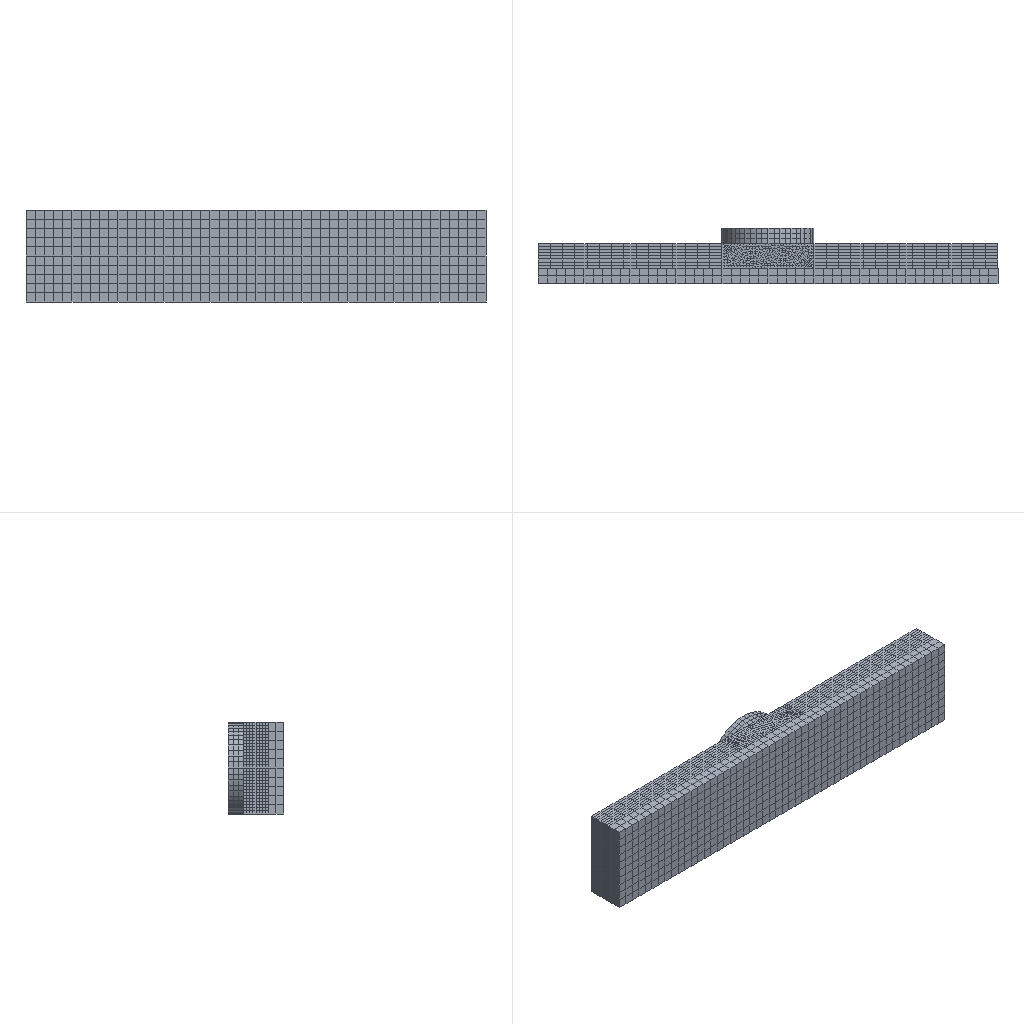Simulation study | abaqus
Set-up summary:
category,name,step,type,value,unit,region
solver,abaqus
solver,version,,,Abaqus/Explicit 2020
units,not stated in the deck,,not stated
analysis,deck,,dynamic temperature-displacement,dynamic temperature-displacement
load_step,Step-1,Step-1,dynamic temperature-displacement
load_step,requested,,,1
mesh,nodes,,,23411
mesh,elements,,,18583
element_type,C3D8RT,,solid,18583
load,load commands in deck,,count,3
bc,support commands in deck,,count,7
material,MATERIAL-1,,in results
material,STEEL,,in results
material,TOOL,,in results
check,setup vs results,,match,"per instance, exact: element labels, types and connectivity; labels of the nodes the elements use; coordinates not compared"
Abaqus input file, long lists of numbers shortened:
*Heading
** Job name: Job-1 Model name: Model-1
** Generated by: Abaqus/CAE 2020
*Preprint, echo=NO, model=NO, history=NO, contact=NO
**
** PARTS
**
*Part, name=Part-1
*Node
      1,  -64.008,  -3.941,          30.
      2,  -64.008,   4.059,          30.
** (10290 more lines like these left out)
*Element, type=C3D8RT
   1,  182, 1582, 3826,  770,    1,   11,  364,   82
   2, 1582, 1583, 3827, 3826,   11,   12,  365,  364
** (8398 more lines like these left out)
*Nset, nset=Set-7, generate
     1,  10292,      1
*Elset, elset=Set-7, generate
    1,  8400,     1
** Section: Section-1
*Solid Section, elset=Set-7, material=Material-1
,
*End Part
**
*Part, name=Part-2
*Node
      1,  -64.008,  -3.941,          30.
      2,  -64.008,   4.059,          30.
** (10290 more lines like these left out)
*Element, type=C3D8RT
   1,  182, 1582, 3826,  770,    1,   11,  364,   82
   2, 1582, 1583, 3827, 3826,   11,   12,  365,  364
** (8398 more lines like these left out)
*Nset, nset=Set-3, generate
     1,  10292,      1
*Elset, elset=Set-3, generate
    1,  8400,     1
** Section: Section-1
*Solid Section, elset=Set-3, material=Material-1
,
*End Part
**
*Part, name=Part-3
*Node
      1,   14.489,           0.,   3.882
      2,   13.858,           0.,   5.74
** (1142 more lines like these left out)
*Element, type=C3D8RT
  1,   79,   22,   44,   74,  365,  308,  330,  360
  2,   22,   79,   49,   21,  308,  365,  335,  307
** (781 more lines like these left out)
*Nset, nset=Set-2, generate
    1,  1144,     1
*Elset, elset=Set-2, generate
   1,  783,    1
** Section: tool
*Solid Section, elset=Set-2, material=tool
,
*End Part
**
*Part, name=Part-4
*Node
      1,         -65.,           0.,          30.
      2,         -65.,          2.5,          30.
** (1681 more lines like these left out)
*Element, type=C3D8RT
   1,   34,   35,   38,   37,    1,    2,    5,    4
   2,   35,   36,   39,   38,    2,    3,    6,    5
** (998 more lines like these left out)
*Nset, nset=Set-3, generate
    1,  1683,     1
*Elset, elset=Set-3, generate
    1,  1000,     1
** Section: steel
*Solid Section, elset=Set-3, material=steel
,
*End Part
**
**
** ASSEMBLY
**
*Assembly, name=Assembly
**
*Instance, name=Part-1-1, part=Part-1
*End Instance
**
*Instance, name=Part-2-1, part=Part-2
   21.984, 0.119,           0.
   21.984, 0.119,           0.,    21.984, 0.119,           1.,         180.
*End Instance
**
*Instance, name=Part-3-1, part=Part-3
10.992,     9.059,          15.
*End Instance
**
*Instance, name=Part-4-1, part=Part-4
0.9919,    -8.941,           0.
*End Instance
**
*Node
      1,   10.992,    9.059,          15.
*Nset, nset=Set-1, instance=Part-1-1
    1,    4,    7,    8,    9,   10,   54,   55,   56,   57,   58,   59,   60,   61,   62,   63
   64,   65,   66,   67,   68,   69,   70,   71,   72,   73,   74,   75,   76,   77,   78,   79
** (88 more lines like these left out)
*Nset, nset=Set-1, instance=Part-2-1
    2,    3,    5,    6,   18,   19,   20,   21,   22,   23,   24,   25,   26,   27,   28,   29
   30,   31,   32,   33,   34,   35,   36,   37,   38,   39,   40,   41,   42,   43,   44,   45
** (29 more lines like these left out)
*Elset, elset=Set-1, instance=Part-1-1
    1,    9,   17,   25,   33,   41,   49,   57,   65,   73,   81,   89,   97,  105,  113,  121
  129,  137,  145,  153,  161,  169,  177,  185,  193,  201,  209,  217,  225,  233,  241,  249
** (83 more lines like these left out)
*Elset, elset=Set-1, instance=Part-2-1, generate
    8,  3600,     8
*Nset, nset=Set-4, instance=Part-1-1, generate
     1,  10292,      1
*Nset, nset=Set-4, instance=Part-2-1, generate
     1,  10292,      1
*Nset, nset=Set-4, instance=Part-4-1, generate
    1,  1683,     1
*Nset, nset=Set-4, instance=Part-3-1, generate
    1,  1144,     1
*Elset, elset=Set-4, instance=Part-1-1, generate
    1,  8400,     1
*Elset, elset=Set-4, instance=Part-2-1, generate
    1,  8400,     1
*Elset, elset=Set-4, instance=Part-4-1, generate
    1,  1000,     1
*Elset, elset=Set-4, instance=Part-3-1, generate
   1,  783,    1
*Nset, nset=Set-5
 1,
*Nset, nset=b_Set-2, instance=Part-3-1, generate
    1,  1144,     1
*Elset, elset=b_Set-2, instance=Part-3-1, generate
   1,  783,    1
*Nset, nset=_PickedSet20, internal
 1,
*Elset, elset=_Surf-8_S5, internal, instance=Part-1-1
  233,  234,  235,  236,  237,  238,  239,  240,  473,  474,  475,  476,  477,  478,  479,  480
  713,  714,  715,  716,  717,  718,  719,  720,  953,  954,  955,  956,  957,  958,  959,  960
** (8 more lines like these left out)
*Elset, elset=_Surf-8_S5, internal, instance=Part-2-1
  233,  234,  235,  236,  237,  238,  239,  240,  473,  474,  475,  476,  477,  478,  479,  480
  713,  714,  715,  716,  717,  718,  719,  720,  953,  954,  955,  956,  957,  958,  959,  960
** (8 more lines like these left out)
*Elset, elset=_Surf-8_S5, internal, instance=Part-4-1
   19,   20,   39,   40,   59,   60,   79,   80,   99,  100,  119,  120,  139,  140,  159,  160
  179,  180,  199,  200,  219,  220,  239,  240,  259,  260,  279,  280,  299,  300,  319,  320
** (5 more lines like these left out)
*Elset, elset=_Surf-8_S5, internal, instance=Part-3-1, generate
  31,  553,  261
*Elset, elset=_Surf-8_S2, internal, instance=Part-1-1
    1,    2,    3,    4,    5,    6,    7,    8,    9,   10,   11,   12,   13,   14,   15,   16
   17,   18,   19,   20,   21,   22,   23,   24,   25,   26,   27,   28,   29,   30,   31,   32
** (23 more lines like these left out)
*Elset, elset=_Surf-8_S2, internal, instance=Part-2-1
    1,    2,    3,    4,    5,    6,    7,    8,    9,   10,   11,   12,   13,   14,   15,   16
   17,   18,   19,   20,   21,   22,   23,   24,   25,   26,   27,   28,   29,   30,   31,   32
** (23 more lines like these left out)
*Elset, elset=_Surf-8_S2, internal, instance=Part-4-1, generate
  1,  20,   1
*Elset, elset=_Surf-8_S2, internal, instance=Part-3-1, generate
 523,  783,    1
*Elset, elset=_Surf-8_S6, internal, instance=Part-1-1
    1,    9,   17,   25,   33,   41,   49,   57,   65,   73,   81,   89,   97,  105,  113,  121
  129,  137,  145,  153,  161,  169,  177,  185,  193,  201,  209,  217,  225,  233,  241,  249
** (120 more lines like these left out)
*Elset, elset=_Surf-8_S6, internal, instance=Part-2-1
    1,    9,   17,   25,   33,   41,   49,   57,   65,   73,   81,   89,   97,  105,  113,  121
  129,  137,  145,  153,  161,  169,  177,  185,  193,  201,  209,  217,  225,  233,  241,  249
** (120 more lines like these left out)
*Elset, elset=_Surf-8_S6, internal, instance=Part-4-1, generate
   1,  999,    2
*Elset, elset=_Surf-8_S6, internal, instance=Part-3-1
   2,   8,   9,  11,  14,  17,  22,  23,  24,  33,  35,  42,  63,  72, 263, 269
 270, 272, 275, 278, 283, 284, 285, 294, 296, 303, 324, 333, 524, 530, 531, 533
** (1 more lines like these left out)
*Elset, elset=_Surf-8_S4, internal, instance=Part-1-1
    8,   16,   24,   32,   40,   48,   56,   64,   72,   80,   88,   96,  104,  112,  120,  128
  136,  144,  152,  160,  168,  176,  184,  192,  200,  208,  216,  224,  232,  240,  248,  256
** (45 more lines like these left out)
*Elset, elset=_Surf-8_S4, internal, instance=Part-2-1
    8,   16,   24,   32,   40,   48,   56,   64,   72,   80,   88,   96,  104,  112,  120,  128
  136,  144,  152,  160,  168,  176,  184,  192,  200,  208,  216,  224,  232,  240,  248,  256
** (45 more lines like these left out)
*Elset, elset=_Surf-8_S4, internal, instance=Part-4-1, generate
    2,  1000,     2
*Elset, elset=_Surf-8_S4, internal, instance=Part-3-1
   1,   3,   4,   5,  10,  12,  13,  15,  19,  25,  26,  29,  34,  36,  38,  39
  41,  43,  44,  45,  46,  47,  48,  49,  51,  53,  56,  58,  61,  68,  80,  96
** (5 more lines like these left out)
*Elset, elset=_Surf-8_S3, internal, instance=Part-1-1
    1,    2,    3,    4,    5,    6,    7,    8,  241,  242,  243,  244,  245,  246,  247,  248
  481,  482,  483,  484,  485,  486,  487,  488,  721,  722,  723,  724,  725,  726,  727,  728
** (12 more lines like these left out)
*Elset, elset=_Surf-8_S3, internal, instance=Part-2-1
    1,    2,    3,    4,    5,    6,    7,    8,  241,  242,  243,  244,  245,  246,  247,  248
  481,  482,  483,  484,  485,  486,  487,  488,  721,  722,  723,  724,  725,  726,  727,  728
** (12 more lines like these left out)
*Elset, elset=_Surf-8_S3, internal, instance=Part-4-1
   1,   2,  21,  22,  41,  42,  61,  62,  81,  82, 101, 102, 121, 122, 141, 142
 161, 162, 181, 182, 201, 202, 221, 222, 241, 242, 261, 262, 281, 282, 301, 302
** (5 more lines like these left out)
*Elset, elset=_Surf-8_S1, internal, instance=Part-1-1, generate
 3601,  3760,     1
*Elset, elset=_Surf-8_S1, internal, instance=Part-2-1, generate
 3601,  3760,     1
*Elset, elset=_Surf-8_S1, internal, instance=Part-4-1, generate
  981,  1000,     1
*Elset, elset=_Surf-8_S1, internal, instance=Part-3-1, generate
   1,  261,    1
*Surface, type=ELEMENT, name=Surf-8
_Surf-8_S5, S5
_Surf-8_S2, S2
_Surf-8_S6, S6
_Surf-8_S4, S4
_Surf-8_S3, S3
_Surf-8_S1, S1
*Elset, elset=_Surf-9_S5, internal, instance=Part-1-1
  233,  234,  235,  236,  237,  238,  239,  240,  473,  474,  475,  476,  477,  478,  479,  480
  713,  714,  715,  716,  717,  718,  719,  720,  953,  954,  955,  956,  957,  958,  959,  960
** (8 more lines like these left out)
*Elset, elset=_Surf-9_S5, internal, instance=Part-2-1
  233,  234,  235,  236,  237,  238,  239,  240,  473,  474,  475,  476,  477,  478,  479,  480
  713,  714,  715,  716,  717,  718,  719,  720,  953,  954,  955,  956,  957,  958,  959,  960
** (8 more lines like these left out)
*Elset, elset=_Surf-9_S5, internal, instance=Part-4-1
   19,   20,   39,   40,   59,   60,   79,   80,   99,  100,  119,  120,  139,  140,  159,  160
  179,  180,  199,  200,  219,  220,  239,  240,  259,  260,  279,  280,  299,  300,  319,  320
** (5 more lines like these left out)
*Elset, elset=_Surf-9_S5, internal, instance=Part-3-1, generate
  31,  553,  261
*Elset, elset=_Surf-9_S2, internal, instance=Part-1-1
    1,    2,    3,    4,    5,    6,    7,    8,    9,   10,   11,   12,   13,   14,   15,   16
   17,   18,   19,   20,   21,   22,   23,   24,   25,   26,   27,   28,   29,   30,   31,   32
** (23 more lines like these left out)
*Elset, elset=_Surf-9_S2, internal, instance=Part-2-1
    1,    2,    3,    4,    5,    6,    7,    8,    9,   10,   11,   12,   13,   14,   15,   16
   17,   18,   19,   20,   21,   22,   23,   24,   25,   26,   27,   28,   29,   30,   31,   32
** (23 more lines like these left out)
*Elset, elset=_Surf-9_S2, internal, instance=Part-4-1, generate
  1,  20,   1
*Elset, elset=_Surf-9_S2, internal, instance=Part-3-1, generate
 523,  783,    1
*Elset, elset=_Surf-9_S6, internal, instance=Part-1-1
    1,    9,   17,   25,   33,   41,   49,   57,   65,   73,   81,   89,   97,  105,  113,  121
  129,  137,  145,  153,  161,  169,  177,  185,  193,  201,  209,  217,  225,  233,  241,  249
** (120 more lines like these left out)
*Elset, elset=_Surf-9_S6, internal, instance=Part-2-1
    1,    9,   17,   25,   33,   41,   49,   57,   65,   73,   81,   89,   97,  105,  113,  121
  129,  137,  145,  153,  161,  169,  177,  185,  193,  201,  209,  217,  225,  233,  241,  249
** (120 more lines like these left out)
*Elset, elset=_Surf-9_S6, internal, instance=Part-4-1, generate
   1,  999,    2
*Elset, elset=_Surf-9_S6, internal, instance=Part-3-1
   2,   8,   9,  11,  14,  17,  22,  23,  24,  33,  35,  42,  63,  72, 263, 269
 270, 272, 275, 278, 283, 284, 285, 294, 296, 303, 324, 333, 524, 530, 531, 533
** (1 more lines like these left out)
*Elset, elset=_Surf-9_S4, internal, instance=Part-1-1
    8,   16,   24,   32,   40,   48,   56,   64,   72,   80,   88,   96,  104,  112,  120,  128
  136,  144,  152,  160,  168,  176,  184,  192,  200,  208,  216,  224,  232,  240,  248,  256
** (45 more lines like these left out)
*Elset, elset=_Surf-9_S4, internal, instance=Part-2-1
    8,   16,   24,   32,   40,   48,   56,   64,   72,   80,   88,   96,  104,  112,  120,  128
  136,  144,  152,  160,  168,  176,  184,  192,  200,  208,  216,  224,  232,  240,  248,  256
** (45 more lines like these left out)
*Elset, elset=_Surf-9_S4, internal, instance=Part-4-1, generate
    2,  1000,     2
*Elset, elset=_Surf-9_S4, internal, instance=Part-3-1
   1,   3,   4,   5,  10,  12,  13,  15,  19,  25,  26,  29,  34,  36,  38,  39
  41,  43,  44,  45,  46,  47,  48,  49,  51,  53,  56,  58,  61,  68,  80,  96
** (5 more lines like these left out)
*Elset, elset=_Surf-9_S3, internal, instance=Part-1-1
    1,    2,    3,    4,    5,    6,    7,    8,  241,  242,  243,  244,  245,  246,  247,  248
  481,  482,  483,  484,  485,  486,  487,  488,  721,  722,  723,  724,  725,  726,  727,  728
** (12 more lines like these left out)
*Elset, elset=_Surf-9_S3, internal, instance=Part-2-1
    1,    2,    3,    4,    5,    6,    7,    8,  241,  242,  243,  244,  245,  246,  247,  248
  481,  482,  483,  484,  485,  486,  487,  488,  721,  722,  723,  724,  725,  726,  727,  728
** (12 more lines like these left out)
*Elset, elset=_Surf-9_S3, internal, instance=Part-4-1
   1,   2,  21,  22,  41,  42,  61,  62,  81,  82, 101, 102, 121, 122, 141, 142
 161, 162, 181, 182, 201, 202, 221, 222, 241, 242, 261, 262, 281, 282, 301, 302
** (5 more lines like these left out)
*Elset, elset=_Surf-9_S1, internal, instance=Part-1-1, generate
 3601,  3760,     1
*Elset, elset=_Surf-9_S1, internal, instance=Part-2-1, generate
 3601,  3760,     1
*Elset, elset=_Surf-9_S1, internal, instance=Part-4-1, generate
  981,  1000,     1
*Elset, elset=_Surf-9_S1, internal, instance=Part-3-1, generate
   1,  261,    1
*Surface, type=ELEMENT, name=Surf-9
_Surf-9_S5, S5
_Surf-9_S2, S2
_Surf-9_S6, S6
_Surf-9_S4, S4
_Surf-9_S3, S3
_Surf-9_S1, S1
*Elset, elset=_m_Surf-1_S4, internal, instance=Part-3-1
   1,   3,   4,   5,  10,  12,  13,  15,  19,  25,  26,  29,  34,  36,  38,  39
  41,  43,  44,  45,  46,  47,  48,  49,  51,  53,  56,  58,  61,  68,  80,  96
** (5 more lines like these left out)
*Elset, elset=_m_Surf-1_S6, internal, instance=Part-3-1
   2,   8,   9,  11,  14,  17,  22,  23,  24,  33,  35,  42,  63,  72, 263, 269
 270, 272, 275, 278, 283, 284, 285, 294, 296, 303, 324, 333, 524, 530, 531, 533
** (1 more lines like these left out)
*Elset, elset=_m_Surf-1_S5, internal, instance=Part-3-1, generate
  31,  553,  261
*Elset, elset=_m_Surf-1_S2, internal, instance=Part-3-1, generate
 523,  783,    1
*Surface, type=ELEMENT, name=m_Surf-1
_m_Surf-1_S4, S4
_m_Surf-1_S6, S6
_m_Surf-1_S2, S2
_m_Surf-1_S5, S5
*Elset, elset=_m_Surf-3_S6, internal, instance=Part-2-1
 3601, 3602, 3603, 3605, 3606, 3607, 3609, 3610, 3612, 3614, 3615, 3622, 3623, 3624, 3625, 3626
 3628, 3632, 3633, 3634, 3679, 3682, 3755, 3761, 3762, 3763, 3765, 3766, 3767, 3769, 3770, 3772
** (42 more lines like these left out)
*Elset, elset=_m_Surf-3_S4, internal, instance=Part-2-1
 3616, 3617, 3627, 3629, 3630, 3631, 3667, 3776, 3777, 3787, 3789, 3790, 3791, 3827, 3936, 3937
 3947, 3949, 3950, 3951, 3987, 4096, 4097, 4107, 4109, 4110, 4111, 4147, 4256, 4257, 4267, 4269
** (12 more lines like these left out)
*Elset, elset=_m_Surf-3_S3, internal, instance=Part-2-1
 3636, 3637, 3687, 3796, 3797, 3847, 3956, 3957, 4007, 4116, 4117, 4167, 4276, 4277, 4327, 4436
 4437, 4487, 4596, 4597, 4647, 4756, 4757, 4807, 4916, 4917, 4967, 5076, 5077, 5127, 5236, 5237
** (4 more lines like these left out)
*Elset, elset=_m_Surf-3_S5, internal, instance=Part-2-1, generate
 3685,  8325,   160
*Surface, type=ELEMENT, name=m_Surf-3
_m_Surf-3_S6, S6
_m_Surf-3_S4, S4
_m_Surf-3_S3, S3
_m_Surf-3_S5, S5
*Elset, elset=_m_Surf-5_S6, internal, instance=Part-1-1
    1,    9,   17,   25,   33,   41,   49,   57,   65,   73,   81,   89,   97,  105,  113,  121
  129,  137,  145,  153,  161,  169,  177,  185,  193,  201,  209,  217,  225,  233,  241,  249
** (77 more lines like these left out)
*Elset, elset=_m_Surf-5_S4, internal, instance=Part-1-1
 3664, 3690, 3699, 3824, 3850, 3859, 3984, 4010, 4019, 4144, 4170, 4179, 4304, 4330, 4339, 4464
 4490, 4499, 4624, 4650, 4659, 4784, 4810, 4819, 4944, 4970, 4979, 5104, 5130, 5139, 5264, 5290
** (4 more lines like these left out)
*Surface, type=ELEMENT, name=m_Surf-5
_m_Surf-5_S6, S6
_m_Surf-5_S4, S4
*Elset, elset=_m_Surf-7_S4, internal, instance=Part-2-1, generate
    8,  3600,     8
*Surface, type=ELEMENT, name=m_Surf-7
_m_Surf-7_S4, S4
*Elset, elset=_s_Surf-1_S6, internal, instance=Part-2-1
 3604, 3608, 3637, 3638, 3643, 3646, 3648, 3649, 3652, 3657, 3661, 3666, 3669, 3670, 3671, 3672
 3673, 3674, 3677, 3678, 3681, 3683, 3684, 3686, 3688, 3691, 3693, 3764, 3768, 3797, 3798, 3803
** (49 more lines like these left out)
*Elset, elset=_s_Surf-1_S4, internal, instance=Part-2-1
 3664, 3690, 3699, 3824, 3850, 3859, 3984, 4010, 4019, 4144, 4170, 4179, 4304, 4330, 4339, 4464
 4490, 4499, 4624, 4650, 4659, 4784, 4810, 4819, 4944, 4970, 4979, 5104, 5130, 5139, 5264, 5290
** (4 more lines like these left out)
*Surface, type=ELEMENT, name=s_Surf-1
_s_Surf-1_S6, S6
_s_Surf-1_S4, S4
*Elset, elset=_s_Surf-3_S6, internal, instance=Part-1-1
 3601, 3602, 3603, 3605, 3606, 3607, 3609, 3610, 3612, 3614, 3615, 3622, 3623, 3624, 3625, 3626
 3628, 3632, 3633, 3634, 3679, 3682, 3755, 3761, 3762, 3763, 3765, 3766, 3767, 3769, 3770, 3772
** (42 more lines like these left out)
*Elset, elset=_s_Surf-3_S4, internal, instance=Part-1-1
 3616, 3617, 3627, 3629, 3630, 3631, 3667, 3776, 3777, 3787, 3789, 3790, 3791, 3827, 3936, 3937
 3947, 3949, 3950, 3951, 3987, 4096, 4097, 4107, 4109, 4110, 4111, 4147, 4256, 4257, 4267, 4269
** (12 more lines like these left out)
*Elset, elset=_s_Surf-3_S3, internal, instance=Part-1-1
 3636, 3637, 3687, 3796, 3797, 3847, 3956, 3957, 4007, 4116, 4117, 4167, 4276, 4277, 4327, 4436
 4437, 4487, 4596, 4597, 4647, 4756, 4757, 4807, 4916, 4917, 4967, 5076, 5077, 5127, 5236, 5237
** (4 more lines like these left out)
*Elset, elset=_s_Surf-3_S5, internal, instance=Part-1-1, generate
 3685,  8325,   160
*Surface, type=ELEMENT, name=s_Surf-3
_s_Surf-3_S6, S6
_s_Surf-3_S4, S4
_s_Surf-3_S3, S3
_s_Surf-3_S5, S5
*Elset, elset=_s_Surf-5_S4, internal, instance=Part-4-1, generate
    2,  1000,     2
*Surface, type=ELEMENT, name=s_Surf-5
_s_Surf-5_S4, S4
** Constraint: Constraint-1
*Rigid Body, ref node=_PickedSet20, elset=b_Set-2, position=CENTER OF MASS
*End Assembly
*Amplitude, name=Amp-1, definition=PERIODIC
1,         125600.,              0.,          0.0025
          6280.,              0.
**
** MATERIALS
**
*Material, name=Material-1
*Conductivity
 0.3,
*Density
 1e-09,
*Elastic
3000., 0.4
*Expansion
 0.0001,
*Specific Heat
 1.7e+09,
*Material, name=steel
*Conductivity
50.,
*Density
 7.8e-09,
*Elastic
210000., 0.3
*Expansion
 1.2e-05,
*Specific Heat
 4.6e+08,
*Material, name=tool
*Conductivity
250.,
*Density
 2.8e-09,
*Elastic
72000., 0.3
*Expansion
 2.32e-05,
*Specific Heat
 8.8e+08,
**
** INTERACTION PROPERTIES
**
*Surface Interaction, name=IntProp-1
*Friction
 0.4,
*Surface Behavior, pressure-overclosure=HARD
**
** PHYSICAL CONSTANTS
**
*Physical Constants, absolute zero=-273., stefan boltzmann=5.67e-08
**
** PREDEFINED FIELDS
**
** Name: Predefined Field-1   Type: Temperature
*Initial Conditions, type=TEMPERATURE
Set-4, 180.
** ----------------------------------------------------------------
**
** STEP: Step-1
**
*Step, name=Step-1, nlgeom=YES
*Dynamic Temperature-displacement, Explicit
, 0.01
*Bulk Viscosity
0.06, 1.2
**
** BOUNDARY CONDITIONS
**
** Name: BC-1 Type: 对称/反对称/完全固定
*Boundary
Set-1, ENCASTRE
** Name: [REDACTED] : Velocity/Angular velocity
*Boundary, amplitude=Amp-1, type=VELOCITY
Set-5, 1, 1
Set-5, 2, 2, -1.
Set-5, 3, 3
Set-5, 4, 4
Set-5, 5, 5
Set-5, 6, 6
**
** INTERACTIONS
**
** Interaction: Int-1
*Contact Pair, interaction=IntProp-1, mechanical constraint=KINEMATIC, cpset=Int-1
m_Surf-1, s_Surf-1
** Interaction: Int-2
*Contact Pair, interaction=IntProp-1, mechanical constraint=KINEMATIC, cpset=Int-2
m_Surf-3, s_Surf-3
** Interaction: Int-3
*Contact Pair, interaction=IntProp-1, mechanical constraint=KINEMATIC, cpset=Int-3
m_Surf-5, s_Surf-5
** Interaction: Int-3-Copy
*Contact Pair, interaction=IntProp-1, mechanical constraint=KINEMATIC, cpset=Int-3-Copy
m_Surf-7, s_Surf-5
** Interaction: Int-5
*Sradiate
Surf-8, R, 180., 0.5
** Interaction: Int-6
*Sfilm
Surf-9, F, 180., 0.001
**
** OUTPUT REQUESTS
**
*Restart, write, number interval=1, time marks=NO
**
** FIELD OUTPUT: F-Output-1
**
*Output, field, number interval=100
*Node Output
A, NT, RF, RFL, U, V
*Element Output, directions=YES
E, HFL, LE, MISES, MISESMAX, PE, PEEQ, PEEQMAX, PEEQT, PEEQVAVG, PEMAG, PEVAVG, S, SVAVG, TEMP
*Contact Output
CSTRESS,
**
** HISTORY OUTPUT: H-Output-1
**
*Output, history, variable=PRESELECT
*End Step
Results summary:
result,step,Step-1,completed,increments=62211 time=0.01/0.01
result,analysis,,,"dynamic temperature-displacement, explict"
result,last_loadstep,,,1
result,primary field,,,"U, NT11"
result,reaction total,,FX,-97.126,model units
result,reaction total,,FY,-3878.707,model units
result,reaction total,,FZ,-5.224,model units